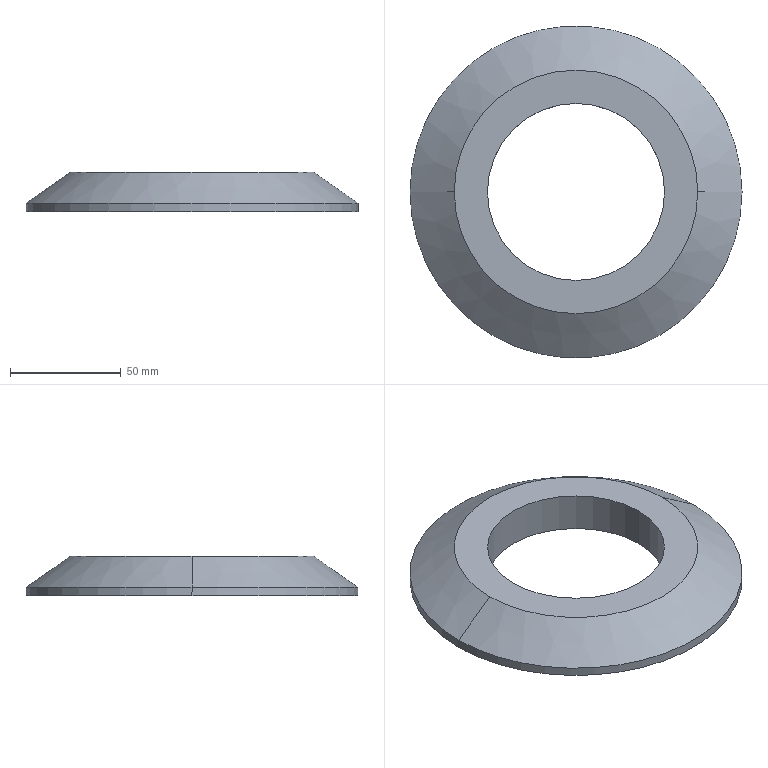Part | STEP file | 1 solid | 8 faces | box 150 x 150 x 18 mm | volume 167499 mm3 | cylinder 4 | plane 2 | cone 2 | commonest cylinder face diameters 80 x2 150 x2
STEP:
#1=CARTESIAN_POINT('',(0.,0.,0.));
#2=DIRECTION('',(0.,0.,1.));
#3=DIRECTION('',(1.,0.,0.));
#4=AXIS2_PLACEMENT_3D('',#1,#2,#3);
#5=CARTESIAN_POINT('',(40.,0.,0.));
#6=VERTEX_POINT('',#5);
#7=CARTESIAN_POINT('',(-40.,0.,0.));
#8=VERTEX_POINT('',#7);
#9=CARTESIAN_POINT('',(0.,0.,0.));
#10=DIRECTION('',(0.,0.,-1.));
#11=DIRECTION('',(1.,0.,0.));
#12=AXIS2_PLACEMENT_3D('',#9,#10,#11);
#13=CIRCLE('',#12,40.);
#14=CARTESIAN_POINT('',(0.,0.,0.));
#15=DIRECTION('',(0.,0.,1.));
#16=DIRECTION('',(1.,0.,0.));
#17=AXIS2_PLACEMENT_3D('',#14,#15,#16);
#18=PLANE('',#17);
#19=CARTESIAN_POINT('',(40.,0.));
#20=CARTESIAN_POINT('',(40.,-69.282));
#21=CARTESIAN_POINT('',(-20.,-34.641));
#22=CARTESIAN_POINT('',(-80.,0.));
#23=CARTESIAN_POINT('',(-20.,34.641));
#24=CARTESIAN_POINT('',(40.,69.282));
#25=CARTESIAN_POINT('',(40.,0.));
#26=(BOUNDED_CURVE()B_SPLINE_CURVE(2,(#19,#20,#21,#22,#23,#24,#25),.UNSPECIFIED.,.T.,.F.)B_SPLINE_CURVE_WITH_KNOTS((1,2,2,2,2,1),(-2.094,0.,2.094,4.189,6.283,8.378),.UNSPECIFIED.)CURVE()GEOMETRIC_REPRESENTATION_ITEM()RATIONAL_B_SPLINE_CURVE((1.,0.5,1.,0.5,1.,0.5,1.))REPRESENTATION_ITEM(''));
#27=(GEOMETRIC_REPRESENTATION_CONTEXT(2)PARAMETRIC_REPRESENTATION_CONTEXT()REPRESENTATION_CONTEXT('',''));
#28=DEFINITIONAL_REPRESENTATION('',(#26),#27);
#29=PCURVE('',#18,#28);
#30=CARTESIAN_POINT('',(0.,0.,-18.));
#31=DIRECTION('',(0.,0.,1.));
#32=DIRECTION('',(1.,0.,0.));
#33=AXIS2_PLACEMENT_3D('',#30,#31,#32);
#34=CYLINDRICAL_SURFACE('',#33,40.);
#35=CARTESIAN_POINT('',(6.283,18.));
#36=DIRECTION('',(-1.,0.));
#37=VECTOR('',#36,1.);
#38=LINE('',#35,#37);
#39=(GEOMETRIC_REPRESENTATION_CONTEXT(2)PARAMETRIC_REPRESENTATION_CONTEXT()REPRESENTATION_CONTEXT('',''));
#40=DEFINITIONAL_REPRESENTATION('',(#38),#39);
#41=PCURVE('',#34,#40);
#42=SURFACE_CURVE('',#13,(#29,#41),.PCURVE_S1.);
#43=EDGE_CURVE('',#6,#8,#42,.T.);
#44=ORIENTED_EDGE('',*,*,#43,.T.);
#45=CARTESIAN_POINT('',(0.,0.,0.));
#46=DIRECTION('',(0.,0.,-1.));
#47=DIRECTION('',(1.,0.,0.));
#48=AXIS2_PLACEMENT_3D('',#45,#46,#47);
#49=CIRCLE('',#48,40.);
#50=CARTESIAN_POINT('',(40.,0.));
#51=CARTESIAN_POINT('',(40.,-69.282));
#52=CARTESIAN_POINT('',(-20.,-34.641));
#53=CARTESIAN_POINT('',(-80.,0.));
#54=CARTESIAN_POINT('',(-20.,34.641));
#55=CARTESIAN_POINT('',(40.,69.282));
#56=CARTESIAN_POINT('',(40.,0.));
#57=(BOUNDED_CURVE()B_SPLINE_CURVE(2,(#50,#51,#52,#53,#54,#55,#56),.UNSPECIFIED.,.T.,.F.)B_SPLINE_CURVE_WITH_KNOTS((1,2,2,2,2,1),(-2.094,0.,2.094,4.189,6.283,8.378),.UNSPECIFIED.)CURVE()GEOMETRIC_REPRESENTATION_ITEM()RATIONAL_B_SPLINE_CURVE((1.,0.5,1.,0.5,1.,0.5,1.))REPRESENTATION_ITEM(''));
#58=(GEOMETRIC_REPRESENTATION_CONTEXT(2)PARAMETRIC_REPRESENTATION_CONTEXT()REPRESENTATION_CONTEXT('',''));
#59=DEFINITIONAL_REPRESENTATION('',(#57),#58);
#60=PCURVE('',#18,#59);
#61=CARTESIAN_POINT('',(0.,0.,-18.));
#62=DIRECTION('',(0.,0.,1.));
#63=DIRECTION('',(1.,0.,0.));
#64=AXIS2_PLACEMENT_3D('',#61,#62,#63);
#65=CYLINDRICAL_SURFACE('',#64,40.);
#66=CARTESIAN_POINT('',(6.283,18.));
#67=DIRECTION('',(-1.,0.));
#68=VECTOR('',#67,1.);
#69=LINE('',#66,#68);
#70=(GEOMETRIC_REPRESENTATION_CONTEXT(2)PARAMETRIC_REPRESENTATION_CONTEXT()REPRESENTATION_CONTEXT('',''));
#71=DEFINITIONAL_REPRESENTATION('',(#69),#70);
#72=PCURVE('',#65,#71);
#73=SURFACE_CURVE('',#49,(#60,#72),.PCURVE_S1.);
#74=EDGE_CURVE('',#8,#6,#73,.T.);
#75=ORIENTED_EDGE('',*,*,#74,.T.);
#76=EDGE_LOOP('',(#44,#75));
#77=FACE_BOUND('',#76,.T.);
#78=CARTESIAN_POINT('',(-55.,0.,0.));
#79=VERTEX_POINT('',#78);
#80=CARTESIAN_POINT('',(55.,0.,0.));
#81=VERTEX_POINT('',#80);
#82=CARTESIAN_POINT('',(0.,0.,0.));
#83=DIRECTION('',(0.,0.,-1.));
#84=DIRECTION('',(-1.,0.,0.));
#85=AXIS2_PLACEMENT_3D('',#82,#83,#84);
#86=CIRCLE('',#85,55.);
#87=CARTESIAN_POINT('',(-55.,0.));
#88=CARTESIAN_POINT('',(-55.,95.263));
#89=CARTESIAN_POINT('',(27.5,47.631));
#90=CARTESIAN_POINT('',(110.,0.));
#91=CARTESIAN_POINT('',(27.5,-47.631));
#92=CARTESIAN_POINT('',(-55.,-95.263));
#93=CARTESIAN_POINT('',(-55.,0.));
#94=(BOUNDED_CURVE()B_SPLINE_CURVE(2,(#87,#88,#89,#90,#91,#92,#93),.UNSPECIFIED.,.T.,.F.)B_SPLINE_CURVE_WITH_KNOTS((1,2,2,2,2,1),(-2.094,0.,2.094,4.189,6.283,8.378),.UNSPECIFIED.)CURVE()GEOMETRIC_REPRESENTATION_ITEM()RATIONAL_B_SPLINE_CURVE((1.,0.5,1.,0.5,1.,0.5,1.))REPRESENTATION_ITEM(''));
#95=(GEOMETRIC_REPRESENTATION_CONTEXT(2)PARAMETRIC_REPRESENTATION_CONTEXT()REPRESENTATION_CONTEXT('',''));
#96=DEFINITIONAL_REPRESENTATION('',(#94),#95);
#97=PCURVE('',#18,#96);
#98=CARTESIAN_POINT('',(0.,0.,-14.));
#99=DIRECTION('',(0.,0.,-1.));
#100=DIRECTION('',(-1.,0.,0.));
#101=AXIS2_PLACEMENT_3D('',#98,#99,#100);
#102=CONICAL_SURFACE('',#101,75.,0.9601);
#103=CARTESIAN_POINT('',(0.,-14.));
#104=DIRECTION('',(1.,0.));
#105=VECTOR('',#104,1.);
#106=LINE('',#103,#105);
#107=(GEOMETRIC_REPRESENTATION_CONTEXT(2)PARAMETRIC_REPRESENTATION_CONTEXT()REPRESENTATION_CONTEXT('',''));
#108=DEFINITIONAL_REPRESENTATION('',(#106),#107);
#109=PCURVE('',#102,#108);
#110=SURFACE_CURVE('',#86,(#97,#109),.PCURVE_S1.);
#111=EDGE_CURVE('',#79,#81,#110,.T.);
#112=ORIENTED_EDGE('',*,*,#111,.F.);
#113=CARTESIAN_POINT('',(0.,0.,0.));
#114=DIRECTION('',(0.,0.,-1.));
#115=DIRECTION('',(-1.,0.,0.));
#116=AXIS2_PLACEMENT_3D('',#113,#114,#115);
#117=CIRCLE('',#116,55.);
#118=CARTESIAN_POINT('',(-55.,0.));
#119=CARTESIAN_POINT('',(-55.,95.263));
#120=CARTESIAN_POINT('',(27.5,47.631));
#121=CARTESIAN_POINT('',(110.,0.));
#122=CARTESIAN_POINT('',(27.5,-47.631));
#123=CARTESIAN_POINT('',(-55.,-95.263));
#124=CARTESIAN_POINT('',(-55.,0.));
#125=(BOUNDED_CURVE()B_SPLINE_CURVE(2,(#118,#119,#120,#121,#122,#123,#124),.UNSPECIFIED.,.T.,.F.)B_SPLINE_CURVE_WITH_KNOTS((1,2,2,2,2,1),(-2.094,0.,2.094,4.189,6.283,8.378),.UNSPECIFIED.)CURVE()GEOMETRIC_REPRESENTATION_ITEM()RATIONAL_B_SPLINE_CURVE((1.,0.5,1.,0.5,1.,0.5,1.))REPRESENTATION_ITEM(''));
#126=(GEOMETRIC_REPRESENTATION_CONTEXT(2)PARAMETRIC_REPRESENTATION_CONTEXT()REPRESENTATION_CONTEXT('',''));
#127=DEFINITIONAL_REPRESENTATION('',(#125),#126);
#128=PCURVE('',#18,#127);
#129=CARTESIAN_POINT('',(0.,0.,-14.));
#130=DIRECTION('',(0.,0.,-1.));
#131=DIRECTION('',(-1.,0.,0.));
#132=AXIS2_PLACEMENT_3D('',#129,#130,#131);
#133=CONICAL_SURFACE('',#132,75.,0.9601);
#134=CARTESIAN_POINT('',(0.,-14.));
#135=DIRECTION('',(1.,0.));
#136=VECTOR('',#135,1.);
#137=LINE('',#134,#136);
#138=(GEOMETRIC_REPRESENTATION_CONTEXT(2)PARAMETRIC_REPRESENTATION_CONTEXT()REPRESENTATION_CONTEXT('',''));
#139=DEFINITIONAL_REPRESENTATION('',(#137),#138);
#140=PCURVE('',#133,#139);
#141=SURFACE_CURVE('',#117,(#128,#140),.PCURVE_S1.);
#142=EDGE_CURVE('',#81,#79,#141,.T.);
#143=ORIENTED_EDGE('',*,*,#142,.F.);
#144=EDGE_LOOP('',(#112,#143));
#145=FACE_BOUND('',#144,.T.);
#146=ADVANCED_FACE('',(#77,#145),#18,.T.);
#147=CARTESIAN_POINT('',(75.,0.,-14.));
#148=VERTEX_POINT('',#147);
#149=CARTESIAN_POINT('',(75.,0.,-14.));
#150=DIRECTION('',(0.8192,0.,-0.5735));
#151=VECTOR('',#150,1.);
#152=LINE('',#149,#151);
#153=CARTESIAN_POINT('',(3.142,0.));
#154=DIRECTION('',(0.,1.));
#155=VECTOR('',#154,1.);
#156=LINE('',#153,#155);
#157=(GEOMETRIC_REPRESENTATION_CONTEXT(2)PARAMETRIC_REPRESENTATION_CONTEXT()REPRESENTATION_CONTEXT('',''));
#158=DEFINITIONAL_REPRESENTATION('',(#156),#157);
#159=PCURVE('',#133,#158);
#160=CARTESIAN_POINT('',(3.142,0.));
#161=DIRECTION('',(0.,1.));
#162=VECTOR('',#161,1.);
#163=LINE('',#160,#162);
#164=(GEOMETRIC_REPRESENTATION_CONTEXT(2)PARAMETRIC_REPRESENTATION_CONTEXT()REPRESENTATION_CONTEXT('',''));
#165=DEFINITIONAL_REPRESENTATION('',(#163),#164);
#166=PCURVE('',#102,#165);
#167=SURFACE_CURVE('',#152,(#159,#166),.PCURVE_S1.);
#168=EDGE_CURVE('',#81,#148,#167,.T.);
#169=ORIENTED_EDGE('',*,*,#168,.F.);
#170=ORIENTED_EDGE('',*,*,#142,.T.);
#171=CARTESIAN_POINT('',(-75.,0.,-14.));
#172=VERTEX_POINT('',#171);
#173=CARTESIAN_POINT('',(-75.,0.,-14.));
#174=DIRECTION('',(-0.8192,0.,-0.5735));
#175=VECTOR('',#174,1.);
#176=LINE('',#173,#175);
#177=CARTESIAN_POINT('',(6.283,0.));
#178=DIRECTION('',(0.,1.));
#179=VECTOR('',#178,1.);
#180=LINE('',#177,#179);
#181=(GEOMETRIC_REPRESENTATION_CONTEXT(2)PARAMETRIC_REPRESENTATION_CONTEXT()REPRESENTATION_CONTEXT('',''));
#182=DEFINITIONAL_REPRESENTATION('',(#180),#181);
#183=PCURVE('',#133,#182);
#184=CARTESIAN_POINT('',(0.,0.));
#185=DIRECTION('',(0.,1.));
#186=VECTOR('',#185,1.);
#187=LINE('',#184,#186);
#188=(GEOMETRIC_REPRESENTATION_CONTEXT(2)PARAMETRIC_REPRESENTATION_CONTEXT()REPRESENTATION_CONTEXT('',''));
#189=DEFINITIONAL_REPRESENTATION('',(#187),#188);
#190=PCURVE('',#102,#189);
#191=SURFACE_CURVE('',#176,(#183,#190),.PCURVE_S1.);
#192=EDGE_CURVE('',#79,#172,#191,.T.);
#193=ORIENTED_EDGE('',*,*,#192,.T.);
#194=CARTESIAN_POINT('',(0.,0.,-14.));
#195=DIRECTION('',(0.,0.,-1.));
#196=DIRECTION('',(1.,0.,0.));
#197=AXIS2_PLACEMENT_3D('',#194,#195,#196);
#198=CIRCLE('',#197,75.);
#199=CARTESIAN_POINT('',(3.142,0.));
#200=DIRECTION('',(1.,0.));
#201=VECTOR('',#200,1.);
#202=LINE('',#199,#201);
#203=(GEOMETRIC_REPRESENTATION_CONTEXT(2)PARAMETRIC_REPRESENTATION_CONTEXT()REPRESENTATION_CONTEXT('',''));
#204=DEFINITIONAL_REPRESENTATION('',(#202),#203);
#205=PCURVE('',#133,#204);
#206=CARTESIAN_POINT('',(0.,0.,-18.));
#207=DIRECTION('',(0.,0.,1.));
#208=DIRECTION('',(1.,0.,0.));
#209=AXIS2_PLACEMENT_3D('',#206,#207,#208);
#210=CYLINDRICAL_SURFACE('',#209,75.);
#211=CARTESIAN_POINT('',(6.283,4.));
#212=DIRECTION('',(-1.,0.));
#213=VECTOR('',#212,1.);
#214=LINE('',#211,#213);
#215=(GEOMETRIC_REPRESENTATION_CONTEXT(2)PARAMETRIC_REPRESENTATION_CONTEXT()REPRESENTATION_CONTEXT('',''));
#216=DEFINITIONAL_REPRESENTATION('',(#214),#215);
#217=PCURVE('',#210,#216);
#218=SURFACE_CURVE('',#198,(#205,#217),.PCURVE_S1.);
#219=EDGE_CURVE('',#148,#172,#218,.T.);
#220=ORIENTED_EDGE('',*,*,#219,.F.);
#221=EDGE_LOOP('',(#169,#170,#193,#220));
#222=FACE_BOUND('',#221,.T.);
#223=ADVANCED_FACE('',(#222),#133,.T.);
#224=ORIENTED_EDGE('',*,*,#74,.T.);
#225=CARTESIAN_POINT('',(40.,0.,-18.));
#226=VERTEX_POINT('',#225);
#227=CARTESIAN_POINT('',(40.,0.,-18.));
#228=DIRECTION('',(0.,0.,1.));
#229=VECTOR('',#228,1.);
#230=LINE('',#227,#229);
#231=CARTESIAN_POINT('',(0.,0.));
#232=DIRECTION('',(0.,1.));
#233=VECTOR('',#232,1.);
#234=LINE('',#231,#233);
#235=(GEOMETRIC_REPRESENTATION_CONTEXT(2)PARAMETRIC_REPRESENTATION_CONTEXT()REPRESENTATION_CONTEXT('',''));
#236=DEFINITIONAL_REPRESENTATION('',(#234),#235);
#237=PCURVE('',#65,#236);
#238=CARTESIAN_POINT('',(6.283,0.));
#239=DIRECTION('',(0.,1.));
#240=VECTOR('',#239,1.);
#241=LINE('',#238,#240);
#242=(GEOMETRIC_REPRESENTATION_CONTEXT(2)PARAMETRIC_REPRESENTATION_CONTEXT()REPRESENTATION_CONTEXT('',''));
#243=DEFINITIONAL_REPRESENTATION('',(#241),#242);
#244=PCURVE('',#34,#243);
#245=SURFACE_CURVE('',#230,(#237,#244),.PCURVE_S1.);
#246=EDGE_CURVE('',#226,#6,#245,.T.);
#247=ORIENTED_EDGE('',*,*,#246,.F.);
#248=CARTESIAN_POINT('',(-40.,0.,-18.));
#249=VERTEX_POINT('',#248);
#250=CARTESIAN_POINT('',(0.,0.,-18.));
#251=DIRECTION('',(0.,0.,1.));
#252=DIRECTION('',(1.,0.,0.));
#253=AXIS2_PLACEMENT_3D('',#250,#251,#252);
#254=CIRCLE('',#253,40.);
#255=CARTESIAN_POINT('',(0.,0.));
#256=DIRECTION('',(1.,0.));
#257=VECTOR('',#256,1.);
#258=LINE('',#255,#257);
#259=(GEOMETRIC_REPRESENTATION_CONTEXT(2)PARAMETRIC_REPRESENTATION_CONTEXT()REPRESENTATION_CONTEXT('',''));
#260=DEFINITIONAL_REPRESENTATION('',(#258),#259);
#261=PCURVE('',#65,#260);
#262=CARTESIAN_POINT('',(0.,0.,-18.));
#263=DIRECTION('',(0.,0.,-1.));
#264=DIRECTION('',(0.,-1.,0.));
#265=AXIS2_PLACEMENT_3D('',#262,#263,#264);
#266=PLANE('',#265);
#267=CARTESIAN_POINT('',(0.,-40.));
#268=CARTESIAN_POINT('',(-69.282,-40.));
#269=CARTESIAN_POINT('',(-34.641,20.));
#270=CARTESIAN_POINT('',(0.,80.));
#271=CARTESIAN_POINT('',(34.641,20.));
#272=CARTESIAN_POINT('',(69.282,-40.));
#273=CARTESIAN_POINT('',(0.,-40.));
#274=(BOUNDED_CURVE()B_SPLINE_CURVE(2,(#267,#268,#269,#270,#271,#272,#273),.UNSPECIFIED.,.T.,.F.)B_SPLINE_CURVE_WITH_KNOTS((1,2,2,2,2,1),(-2.094,0.,2.094,4.189,6.283,8.378),.UNSPECIFIED.)CURVE()GEOMETRIC_REPRESENTATION_ITEM()RATIONAL_B_SPLINE_CURVE((1.,0.5,1.,0.5,1.,0.5,1.))REPRESENTATION_ITEM(''));
#275=(GEOMETRIC_REPRESENTATION_CONTEXT(2)PARAMETRIC_REPRESENTATION_CONTEXT()REPRESENTATION_CONTEXT('',''));
#276=DEFINITIONAL_REPRESENTATION('',(#274),#275);
#277=PCURVE('',#266,#276);
#278=SURFACE_CURVE('',#254,(#261,#277),.PCURVE_S1.);
#279=EDGE_CURVE('',#226,#249,#278,.T.);
#280=ORIENTED_EDGE('',*,*,#279,.T.);
#281=CARTESIAN_POINT('',(-40.,0.,-18.));
#282=DIRECTION('',(0.,0.,1.));
#283=VECTOR('',#282,1.);
#284=LINE('',#281,#283);
#285=CARTESIAN_POINT('',(3.142,0.));
#286=DIRECTION('',(0.,1.));
#287=VECTOR('',#286,1.);
#288=LINE('',#285,#287);
#289=(GEOMETRIC_REPRESENTATION_CONTEXT(2)PARAMETRIC_REPRESENTATION_CONTEXT()REPRESENTATION_CONTEXT('',''));
#290=DEFINITIONAL_REPRESENTATION('',(#288),#289);
#291=PCURVE('',#65,#290);
#292=CARTESIAN_POINT('',(3.142,0.));
#293=DIRECTION('',(0.,1.));
#294=VECTOR('',#293,1.);
#295=LINE('',#292,#294);
#296=(GEOMETRIC_REPRESENTATION_CONTEXT(2)PARAMETRIC_REPRESENTATION_CONTEXT()REPRESENTATION_CONTEXT('',''));
#297=DEFINITIONAL_REPRESENTATION('',(#295),#296);
#298=PCURVE('',#34,#297);
#299=SURFACE_CURVE('',#284,(#291,#298),.PCURVE_S1.);
#300=EDGE_CURVE('',#249,#8,#299,.T.);
#301=ORIENTED_EDGE('',*,*,#300,.T.);
#302=EDGE_LOOP('',(#224,#247,#280,#301));
#303=FACE_BOUND('',#302,.F.);
#304=ADVANCED_FACE('',(#303),#65,.F.);
#305=CARTESIAN_POINT('',(-75.,0.,-18.));
#306=VERTEX_POINT('',#305);
#307=CARTESIAN_POINT('',(-75.,0.,-18.));
#308=DIRECTION('',(0.,0.,1.));
#309=VECTOR('',#308,1.);
#310=LINE('',#307,#309);
#311=CARTESIAN_POINT('',(3.142,0.));
#312=DIRECTION('',(0.,1.));
#313=VECTOR('',#312,1.);
#314=LINE('',#311,#313);
#315=(GEOMETRIC_REPRESENTATION_CONTEXT(2)PARAMETRIC_REPRESENTATION_CONTEXT()REPRESENTATION_CONTEXT('',''));
#316=DEFINITIONAL_REPRESENTATION('',(#314),#315);
#317=PCURVE('',#210,#316);
#318=CARTESIAN_POINT('',(0.,0.,-18.));
#319=DIRECTION('',(0.,0.,1.));
#320=DIRECTION('',(1.,0.,0.));
#321=AXIS2_PLACEMENT_3D('',#318,#319,#320);
#322=CYLINDRICAL_SURFACE('',#321,75.);
#323=CARTESIAN_POINT('',(3.142,0.));
#324=DIRECTION('',(0.,1.));
#325=VECTOR('',#324,1.);
#326=LINE('',#323,#325);
#327=(GEOMETRIC_REPRESENTATION_CONTEXT(2)PARAMETRIC_REPRESENTATION_CONTEXT()REPRESENTATION_CONTEXT('',''));
#328=DEFINITIONAL_REPRESENTATION('',(#326),#327);
#329=PCURVE('',#322,#328);
#330=SURFACE_CURVE('',#310,(#317,#329),.PCURVE_S1.);
#331=EDGE_CURVE('',#306,#172,#330,.T.);
#332=ORIENTED_EDGE('',*,*,#331,.F.);
#333=CARTESIAN_POINT('',(75.,0.,-18.));
#334=VERTEX_POINT('',#333);
#335=CARTESIAN_POINT('',(0.,0.,-18.));
#336=DIRECTION('',(0.,0.,-1.));
#337=DIRECTION('',(1.,0.,0.));
#338=AXIS2_PLACEMENT_3D('',#335,#336,#337);
#339=CIRCLE('',#338,75.);
#340=CARTESIAN_POINT('',(6.283,0.));
#341=DIRECTION('',(-1.,0.));
#342=VECTOR('',#341,1.);
#343=LINE('',#340,#342);
#344=(GEOMETRIC_REPRESENTATION_CONTEXT(2)PARAMETRIC_REPRESENTATION_CONTEXT()REPRESENTATION_CONTEXT('',''));
#345=DEFINITIONAL_REPRESENTATION('',(#343),#344);
#346=PCURVE('',#210,#345);
#347=CARTESIAN_POINT('',(0.,0.));
#348=DIRECTION('',(0.,-1.));
#349=AXIS2_PLACEMENT_2D('',#347,#348);
#350=CIRCLE('',#349,75.);
#351=(GEOMETRIC_REPRESENTATION_CONTEXT(2)PARAMETRIC_REPRESENTATION_CONTEXT()REPRESENTATION_CONTEXT('',''));
#352=DEFINITIONAL_REPRESENTATION('',(#350),#351);
#353=PCURVE('',#266,#352);
#354=SURFACE_CURVE('',#339,(#346,#353),.PCURVE_S1.);
#355=EDGE_CURVE('',#334,#306,#354,.T.);
#356=ORIENTED_EDGE('',*,*,#355,.F.);
#357=CARTESIAN_POINT('',(75.,0.,-18.));
#358=DIRECTION('',(0.,0.,1.));
#359=VECTOR('',#358,1.);
#360=LINE('',#357,#359);
#361=CARTESIAN_POINT('',(6.283,0.));
#362=DIRECTION('',(0.,1.));
#363=VECTOR('',#362,1.);
#364=LINE('',#361,#363);
#365=(GEOMETRIC_REPRESENTATION_CONTEXT(2)PARAMETRIC_REPRESENTATION_CONTEXT()REPRESENTATION_CONTEXT('',''));
#366=DEFINITIONAL_REPRESENTATION('',(#364),#365);
#367=PCURVE('',#210,#366);
#368=CARTESIAN_POINT('',(0.,0.));
#369=DIRECTION('',(0.,1.));
#370=VECTOR('',#369,1.);
#371=LINE('',#368,#370);
#372=(GEOMETRIC_REPRESENTATION_CONTEXT(2)PARAMETRIC_REPRESENTATION_CONTEXT()REPRESENTATION_CONTEXT('',''));
#373=DEFINITIONAL_REPRESENTATION('',(#371),#372);
#374=PCURVE('',#322,#373);
#375=SURFACE_CURVE('',#360,(#367,#374),.PCURVE_S1.);
#376=EDGE_CURVE('',#334,#148,#375,.T.);
#377=ORIENTED_EDGE('',*,*,#376,.T.);
#378=ORIENTED_EDGE('',*,*,#219,.T.);
#379=EDGE_LOOP('',(#332,#356,#377,#378));
#380=FACE_BOUND('',#379,.T.);
#381=ADVANCED_FACE('',(#380),#210,.T.);
#382=ORIENTED_EDGE('',*,*,#279,.T.);
#383=CARTESIAN_POINT('',(0.,0.,-18.));
#384=DIRECTION('',(0.,0.,1.));
#385=DIRECTION('',(1.,0.,0.));
#386=AXIS2_PLACEMENT_3D('',#383,#384,#385);
#387=CIRCLE('',#386,40.);
#388=CARTESIAN_POINT('',(0.,-40.));
#389=CARTESIAN_POINT('',(-69.282,-40.));
#390=CARTESIAN_POINT('',(-34.641,20.));
#391=CARTESIAN_POINT('',(0.,80.));
#392=CARTESIAN_POINT('',(34.641,20.));
#393=CARTESIAN_POINT('',(69.282,-40.));
#394=CARTESIAN_POINT('',(0.,-40.));
#395=(BOUNDED_CURVE()B_SPLINE_CURVE(2,(#388,#389,#390,#391,#392,#393,#394),.UNSPECIFIED.,.T.,.F.)B_SPLINE_CURVE_WITH_KNOTS((1,2,2,2,2,1),(-2.094,0.,2.094,4.189,6.283,8.378),.UNSPECIFIED.)CURVE()GEOMETRIC_REPRESENTATION_ITEM()RATIONAL_B_SPLINE_CURVE((1.,0.5,1.,0.5,1.,0.5,1.))REPRESENTATION_ITEM(''));
#396=(GEOMETRIC_REPRESENTATION_CONTEXT(2)PARAMETRIC_REPRESENTATION_CONTEXT()REPRESENTATION_CONTEXT('',''));
#397=DEFINITIONAL_REPRESENTATION('',(#395),#396);
#398=PCURVE('',#266,#397);
#399=CARTESIAN_POINT('',(0.,0.));
#400=DIRECTION('',(1.,0.));
#401=VECTOR('',#400,1.);
#402=LINE('',#399,#401);
#403=(GEOMETRIC_REPRESENTATION_CONTEXT(2)PARAMETRIC_REPRESENTATION_CONTEXT()REPRESENTATION_CONTEXT('',''));
#404=DEFINITIONAL_REPRESENTATION('',(#402),#403);
#405=PCURVE('',#34,#404);
#406=SURFACE_CURVE('',#387,(#398,#405),.PCURVE_S1.);
#407=EDGE_CURVE('',#249,#226,#406,.T.);
#408=ORIENTED_EDGE('',*,*,#407,.T.);
#409=EDGE_LOOP('',(#382,#408));
#410=FACE_BOUND('',#409,.T.);
#411=ORIENTED_EDGE('',*,*,#355,.T.);
#412=CARTESIAN_POINT('',(0.,0.,-18.));
#413=DIRECTION('',(0.,0.,-1.));
#414=DIRECTION('',(1.,0.,0.));
#415=AXIS2_PLACEMENT_3D('',#412,#413,#414);
#416=CIRCLE('',#415,75.);
#417=CARTESIAN_POINT('',(0.,0.));
#418=DIRECTION('',(0.,-1.));
#419=AXIS2_PLACEMENT_2D('',#417,#418);
#420=CIRCLE('',#419,75.);
#421=(GEOMETRIC_REPRESENTATION_CONTEXT(2)PARAMETRIC_REPRESENTATION_CONTEXT()REPRESENTATION_CONTEXT('',''));
#422=DEFINITIONAL_REPRESENTATION('',(#420),#421);
#423=PCURVE('',#266,#422);
#424=CARTESIAN_POINT('',(6.283,0.));
#425=DIRECTION('',(-1.,0.));
#426=VECTOR('',#425,1.);
#427=LINE('',#424,#426);
#428=(GEOMETRIC_REPRESENTATION_CONTEXT(2)PARAMETRIC_REPRESENTATION_CONTEXT()REPRESENTATION_CONTEXT('',''));
#429=DEFINITIONAL_REPRESENTATION('',(#427),#428);
#430=PCURVE('',#322,#429);
#431=SURFACE_CURVE('',#416,(#423,#430),.PCURVE_S1.);
#432=EDGE_CURVE('',#306,#334,#431,.T.);
#433=ORIENTED_EDGE('',*,*,#432,.T.);
#434=EDGE_LOOP('',(#411,#433));
#435=FACE_BOUND('',#434,.T.);
#436=ADVANCED_FACE('',(#410,#435),#266,.T.);
#437=ORIENTED_EDGE('',*,*,#111,.T.);
#438=ORIENTED_EDGE('',*,*,#168,.T.);
#439=CARTESIAN_POINT('',(0.,0.,-14.));
#440=DIRECTION('',(0.,0.,-1.));
#441=DIRECTION('',(1.,0.,0.));
#442=AXIS2_PLACEMENT_3D('',#439,#440,#441);
#443=CIRCLE('',#442,75.);
#444=CARTESIAN_POINT('',(-3.142,0.));
#445=DIRECTION('',(1.,0.));
#446=VECTOR('',#445,1.);
#447=LINE('',#444,#446);
#448=(GEOMETRIC_REPRESENTATION_CONTEXT(2)PARAMETRIC_REPRESENTATION_CONTEXT()REPRESENTATION_CONTEXT('',''));
#449=DEFINITIONAL_REPRESENTATION('',(#447),#448);
#450=PCURVE('',#102,#449);
#451=CARTESIAN_POINT('',(6.283,4.));
#452=DIRECTION('',(-1.,0.));
#453=VECTOR('',#452,1.);
#454=LINE('',#451,#453);
#455=(GEOMETRIC_REPRESENTATION_CONTEXT(2)PARAMETRIC_REPRESENTATION_CONTEXT()REPRESENTATION_CONTEXT('',''));
#456=DEFINITIONAL_REPRESENTATION('',(#454),#455);
#457=PCURVE('',#322,#456);
#458=SURFACE_CURVE('',#443,(#450,#457),.PCURVE_S1.);
#459=EDGE_CURVE('',#172,#148,#458,.T.);
#460=ORIENTED_EDGE('',*,*,#459,.F.);
#461=ORIENTED_EDGE('',*,*,#192,.F.);
#462=EDGE_LOOP('',(#437,#438,#460,#461));
#463=FACE_BOUND('',#462,.T.);
#464=ADVANCED_FACE('',(#463),#102,.T.);
#465=ORIENTED_EDGE('',*,*,#246,.T.);
#466=ORIENTED_EDGE('',*,*,#43,.T.);
#467=ORIENTED_EDGE('',*,*,#300,.F.);
#468=ORIENTED_EDGE('',*,*,#407,.T.);
#469=EDGE_LOOP('',(#465,#466,#467,#468));
#470=FACE_BOUND('',#469,.F.);
#471=ADVANCED_FACE('',(#470),#34,.F.);
#472=ORIENTED_EDGE('',*,*,#432,.F.);
#473=ORIENTED_EDGE('',*,*,#331,.T.);
#474=ORIENTED_EDGE('',*,*,#459,.T.);
#475=ORIENTED_EDGE('',*,*,#376,.F.);
#476=EDGE_LOOP('',(#472,#473,#474,#475));
#477=FACE_BOUND('',#476,.T.);
#478=ADVANCED_FACE('',(#477),#322,.T.);
#479=CLOSED_SHELL('',(#146,#223,#304,#381,#436,#464,#471,#478));
#480=MANIFOLD_SOLID_BREP('',#479);
#481=(LENGTH_UNIT()NAMED_UNIT(*)SI_UNIT(.MILLI.,.METRE.));
#482=UNCERTAINTY_MEASURE_WITH_UNIT(LENGTH_MEASURE(0.0000001),#481,'','');
#483=(NAMED_UNIT(*)PLANE_ANGLE_UNIT()SI_UNIT($,.RADIAN.));
#484=(NAMED_UNIT(*)SI_UNIT($,.STERADIAN.)SOLID_ANGLE_UNIT());
#485=(GEOMETRIC_REPRESENTATION_CONTEXT(3)GLOBAL_UNCERTAINTY_ASSIGNED_CONTEXT((#482))GLOBAL_UNIT_ASSIGNED_CONTEXT((#481,#483,#484))REPRESENTATION_CONTEXT('',''));
#486=ADVANCED_BREP_SHAPE_REPRESENTATION('',(#4,#480),#485);